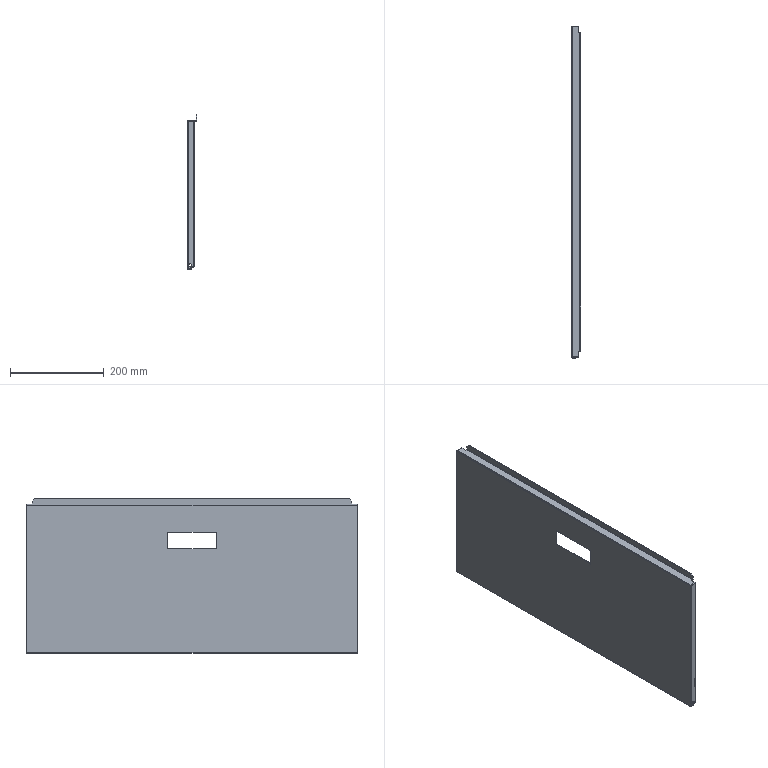Part | SolidWorks | features EdgeFlange 6, ICE 5, Chamfer 1, FlatPattern 1, SMBaseFlange 1, SheetMetal 1 | 1 solid | 96 faces | box 20.237 x 707 x 329 mm | volume 397548 mm3 | plane 76 | cylinder 20 | commonest cylinder face diameters 0.6 x6 3.6 x6 7 x4 1.473 x2 4.473 x2